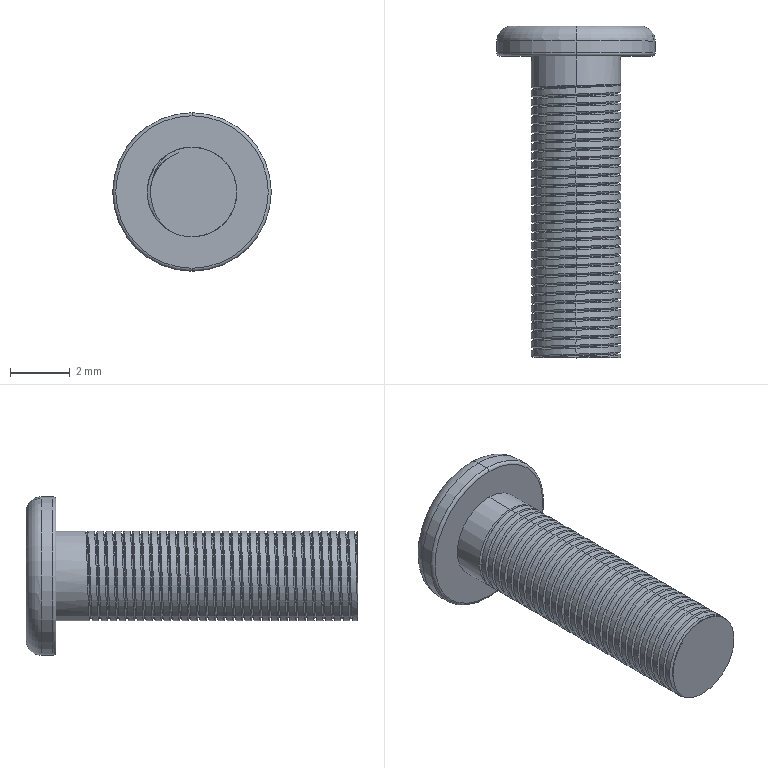Part | SolidWorks | features Fillet 2, Helix 2, ICE 2, SweepCut 2, Extrusion 1 | 1 solid | 91 faces | box 5.3 x 11.1 x 5.3 mm | volume 89.179 mm3 | cylinder 65 | plane 16 | spline 6 | torus 4 | commonest cylinder face diameters 3 x63 5.3 x2